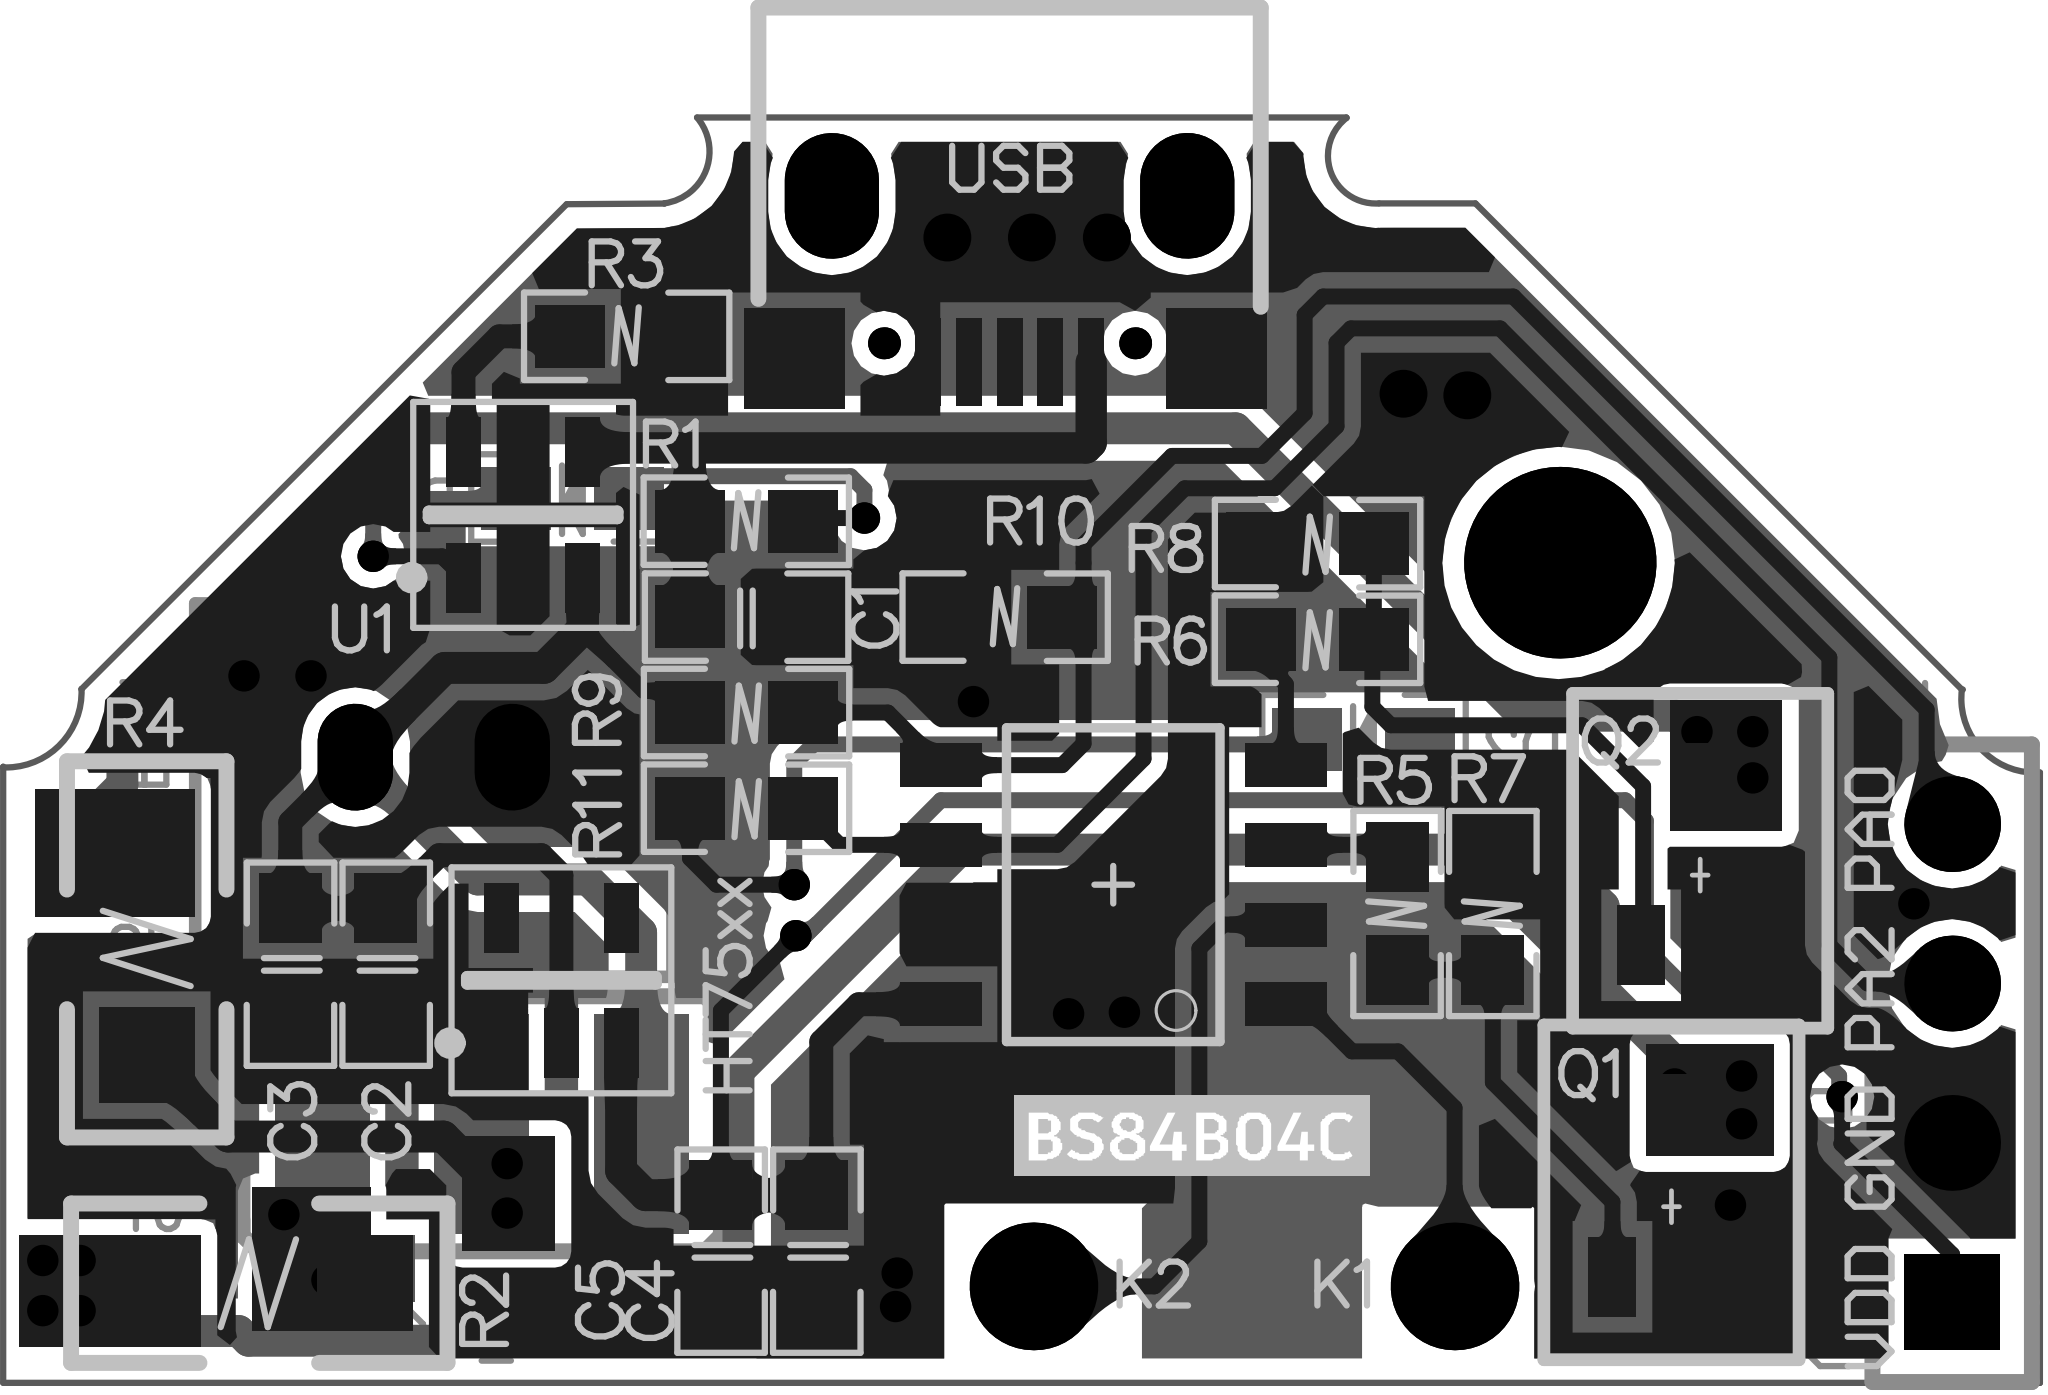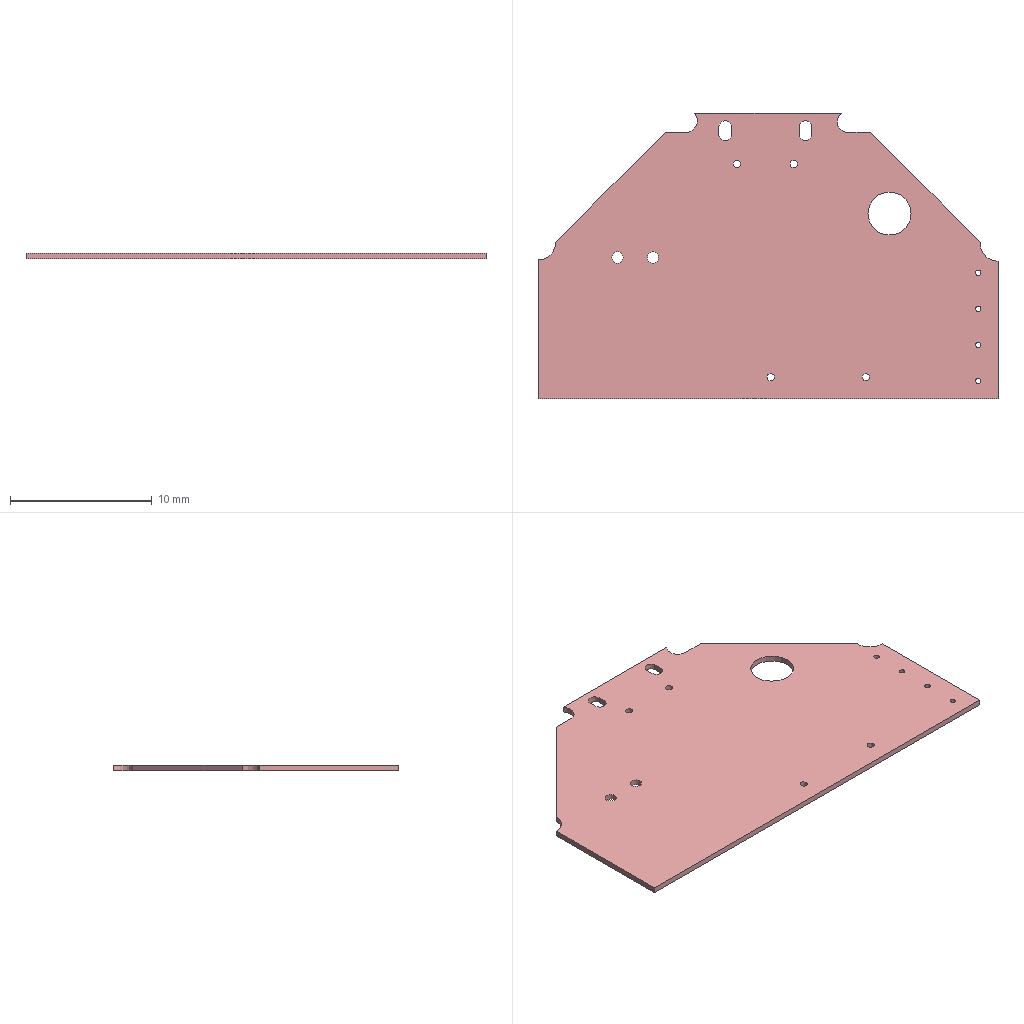Circuit board layout | Altium Designer | box 32.4 x 20.2 x 0.4 mm
Layer stack:
# Altium Designer layer stack of  (unit mm; dielectric type: 0 none, 1 core, 2 prepreg, 3 surface material)
index,name,kind,layer,copper_thickness_mm,dielectric_type,dielectric_thickness_mm,dielectric_material,dielectric_constant
0,Top Paste,other,,,,,,
1,Top Overlay,other,,,,,,
2,Top Solder,dielectric,,,3,0.0102,Solder Resist,3.5
3,Top Layer,copper,Top Layer,0.0356,,,,
4,Dielectric1,dielectric,,,0,0.32,FR-4,4.8
5,Bottom Layer,copper,Bottom Layer,0.0356,,,,
6,Bottom Solder,dielectric,,,3,0.0102,Solder Resist,3.5
7,Bottom Overlay,other,,,,,,
8,Bottom Paste,other,,,,,,
# drill layer pairs: low layer,high layer
drill_pair,Top Layer,Bottom Layer
Part placement:
Designator,Comment,Layer,Footprint,Center-X(mm),Center-Y(mm),Rotation
ICP1,HDR 1X4,BottomLayer,HDR_1x4(2.54),31.039,5.029,90
USB,Comment,TopLayer,Mcro_USB,15.964,17.526,180
HT75xx,HT7530,TopLayer,SOT23_PIN-5,8.89,6.35,90
C1,,TopLayer,C_0603,11.836,12.141,0
C2,,TopLayer,C_0603,6.096,6.604,90
C3,,TopLayer,C_0603,4.572,6.604,90
C4,,TopLayer,C_0603,12.954,2.032,90
C5,,TopLayer,C_0603,11.43,2.032,90
J1,HDR 1X3_2,BottomLayer,º¸±P,7.62,4.064,0
Q1,SS8050,TopLayer,SOT23_BJT_NPN,26.556,2.921,0
Q2,SS8050,TopLayer,SOT23_BJT_NPN,27.013,8.204,0
R1,1K,TopLayer,R_0603,11.836,13.665,180
R2,2R0,TopLayer,R_1206,4.064,1.524,0
R3,2K,TopLayer,R_0603,9.931,16.612,180
R4,2R0,TopLayer,R_1206,2.286,6.858,270
R5,1K,TopLayer,R_0603,22.2,7.417,270
R6,1K,TopLayer,R_0603,20.93,11.786,0
R7,1K,TopLayer,R_0603,23.724,7.417,270
R8,1K,TopLayer,R_0603,20.93,13.31,0
R9,510K,TopLayer,R_0603,11.836,10.617,0
R10,510K,TopLayer,R_0603,15.959,12.137,180
R11,1K,TopLayer,R_0603,11.836,9.093,0
U1,2KAX,TopLayer,SOT23_PIN-5,8.28,13.767,90
U2,BS84B04C,TopLayer,SOP8,17.678,7.874,90
J2,,BottomLayer,HDR_1X2_Pitch_2.5mm,6.858,9.906,0
K1,SN1,TopLayer,KEY,23.114,1.473,0
K2,SN1,TopLayer,KEY,16.408,1.473,0
D1,,BottomLayer,LED_0603,9.068,14.021,180
D2,,BottomLayer,LED_0603,21.666,10.185,180
Pad and via stacks:
# Altium Designer via and pad stacks of  (unit mm). Each distinct definition once, with the count of objects using it.
# via: kind,start_layer,end_layer,hole_mm,diameter_mm,mode(0 simple;1 top-mid-bottom;2 full stack),diameter_per_layer,count,example_net
# pad: kind,layer,hole_mm,hole_type(0 round;1 square;2 slot),plating,top_size,top_shape(1 round;2 rect;3 octagon;9 rounded rect),mid_size,bottom_size,mode,footprint,size_per_layer,count,example
pad,Top Layer,0,0,plated,0.55x1.1,2,0.55x1.1,0.55x1.1,0,SOT23 PIN-5,,10,HT75xx.1
pad,Top Layer,0,0,plated,1.6x1.6,2,1.6x1.6,1.6x1.6,0,Mcro_USB,,2,USB.6
pad,Top Layer,0,0,plated,0.4x1.4,2,0.4x1.4,0.4x1.4,0,Mcro_USB,,5,USB.1
pad,Top Layer,0,0,plated,1.1x1,2,1.1x1,1.1x1,0,C 0603,,10,C1.1
pad,Top Layer,0,0,plated,1.27x0.762,2,1.27x0.762,1.27x0.762,0,SOT23_BJT_NPN,,6,Q1.1
pad,Top Layer,0,0,plated,1.1x1,2,1.1x1,1.1x1,0,R 0603,,18,R1.2
pad,Top Layer,0,0,plated,1.524x1.524,2,1.524x1.524,1.524x1.524,0,R 1206,,4,R2.2
pad,Top Layer,0,0,plated,0.7x1.3,2,0.7x1.3,0.7x1.3,0,SOP8,,8,U2.5
pad,Multi-Layer,0.508,0,plated,2.032x2.032,1,2.032x2.032,2.032x2.032,0,KEY,,2,K2.1
pad,Multi-Layer,3.048,0,plated,3.048x3.048,1,3.048x3.048,3.048x3.048,0,,,1,0
pad,Multi-Layer,0.9,2,plated,2x1.5,1,2x1.5,2x1.5,0,Mcro_USB,,2,USB.9
pad,Multi-Layer,0.508,0,plated,0.508x0.508,1,0.508x0.508,0.508x0.508,0,Mcro_USB,,2,USB.0
pad,Multi-Layer,0.8,0,plated,1.2x1.7,1,1.2x1.7,1.2x1.7,0,HDR 1X2 Pitch 2.5mm,,2,J2.1
pad,Multi-Layer,0.381,0,plated,1.524x1.524,2,1.524x1.524,1.524x1.524,0,HDR 1x4(2.54),,1,ICP1.1
pad,Multi-Layer,0.381,0,plated,1.524x1.524,1,1.524x1.524,1.524x1.524,0,HDR 1x4(2.54),,3,ICP1.2
pad,Bottom Layer,0,0,plated,1.5x3.5,2,1.5x3.5,1.5x3.5,0,\u00BA\u00B8\u00B1P,,3,J1.3
pad,Bottom Layer,0,0,plated,1.1x1,2,1.1x1,1.1x1,0,LED_0603,,4,D1.2
via,Top Layer,Bottom Layer,0.3,0.5,0,,35,NetD2_2
via,Top Layer,Bottom Layer,0.508,0.762,0,,5,GND
Copper pours:
name,layer,net,type(0 solid;1 hatched;2 none)
Keep-Out Layer-No Net,Bottom Layer,GND,0
Top Layer-No Net 1,Top Layer,GND,0
Design rules, without the lines most boards share:
# Altium Designer design rules of  (exported by Altium Designer, unit mm)
# columns: name | kind | enabled | priority | scope1 | scope2 | descriptor | typed fields (field=value)
PolygonConnect_1 | 20 | enabled | 1 | All | All | Polygon Connect Rule(Direct Connect )(Conductor Width=0.254mm) (Relief Angle=90 Angle) (Entries=4) (Air Gap Width=0.254mm) (All),(All) | connect_style(0=relief,1=direct,2=none)=1 relief_conductor_width=0.254 relief_entries=4
Clearance_1 | 0 | enabled | 1 | All | All | Clearance Constraint (Gap=0.254mm) (All),(All) | gap=0.254
ComponentClearance_2 | 24 | enabled | 3 | All | All | Component Clearance Constraint ( Horizontal Gap = 0.508mm, Vertical Gap = 0.508mm ) (All),(All)  | gap=0.508
ComponentClearance_1 | 24 | enabled | 2 | All | All | Component Clearance Constraint ( Horizontal Gap = 0.254mm, Vertical Gap = 0.254mm ) (All),(All)  | gap=0.254
NetAntennae | 56 | enabled | 1 | All | All | Net Antennae (Tolerance=0mm) (All) |
SilkToSilkClearance | 55 | enabled | 1 | All | All | Silk to Silk (Clearance=0.254mm) (All),(All) |
SilkToSolderMaskClearance | 54 | enabled | 1 | IsPad | All | Silk To Solder Mask (Clearance=0.254mm) (IsPad),(All) |
MinimumSolderMaskSliver | 53 | enabled | 1 | All | All | Minimum Solder Mask Sliver (Gap=0.254mm) (All),(All) |
HoleToHoleClearance | 52 | enabled | 1 | All | All | Hole To Hole Clearance (Gap=0.254mm) (All),(All) | gap=0.254
DiffPairsRouting | 51 | enabled | 1 | All | All | Differential Pairs Uncoupled Length using the Gap Constraints (Min=0.254mm) (Max=0.254mm) (Prefered=0.254mm)  and Width Constraints (Min=0.381mm) (Max=0.381mm) (Prefered=0.381mm) (All) |
HoleSize | 42 | enabled | 1 | All | All | Hole Size Constraint (Min=0.025mm) (Max=2.54mm) (All) |
Height | 50 | enabled | 1 | All | All | Height Constraint (Min=0mm) (Max=25.4mm) (Prefered=12.7mm) (All) | min_height=0 max_height=25.4
ComponentClearance | 24 | enabled | 1 | All | All | Component Clearance Constraint ( Horizontal Gap = 0.254mm, Vertical Gap = 0.254mm ) (All),(All)  | gap=0.254
SolderMaskExpansion | 13 | enabled | 1 | All | All | Solder Mask Expansion (Expansion =0.102mm) (All) | expansion=0.1016
PasteMaskExpansion | 14 | enabled | 1 | All | All | Paste Mask Expansion (Expansion =0mm) (All) | expansion=0
RoutingVias | 11 | enabled | 1 | All | All | Routing Via (MinHoleWidth=0.711mm) (MaxHoleWidth=0.711mm) (PreferredHoleWidth=0.711mm) (MinWidth=1.27mm) (MaxWidth=1.27mm) (PreferedWidth=1.27mm) (All) | via_min_hole=0.7112 via_max_hole=0.7112 via_preferred_diameter=1.27 via_preferred_hole=0.7112
RoutingCorners | 10 | enabled | 1 | All | All | Routing Corners (Style=45-Degree) (Min Setback=2.54mm) (Max Setback=2.54mm) (All) |
Width | 2 | enabled | 1 | All | All | Width Constraint (Min=0.254mm) (Max=2.54mm) (Preferred=0.254mm) (All) |
PolygonConnect | 20 | disabled | 2 | IsVia | IsVia | Polygon Connect Rule(Direct Connect )(Conductor Width=0.254mm) (Relief Angle=90 Angle) (Entries=4) (Air Gap Width=0.254mm) (Disabled)(IsVia),(IsVia) | connect_style(0=relief,1=direct,2=none)=1 relief_conductor_width=0.254 relief_entries=4
PlaneClearance | 12 | enabled | 1 | All | All | Power Plane Clearance (Clearance =0.508mm) (All) | clearance=0.508
Clearance | 0 | enabled | 2 | All | All | Clearance Constraint (Gap=0.254mm) (All),(All) | gap=0.254
PlaneConnect_1 | 6 | enabled | 1 | All | All | Power Plane Connect Rule(Relief Connect )(Expansion=0.508mm) (Conductor Width=0.254mm) (Air Gap=0.254mm) (Entries=4) (All) | relief_conductor_width=0.254 relief_entries=4 relief_expansion=0.508